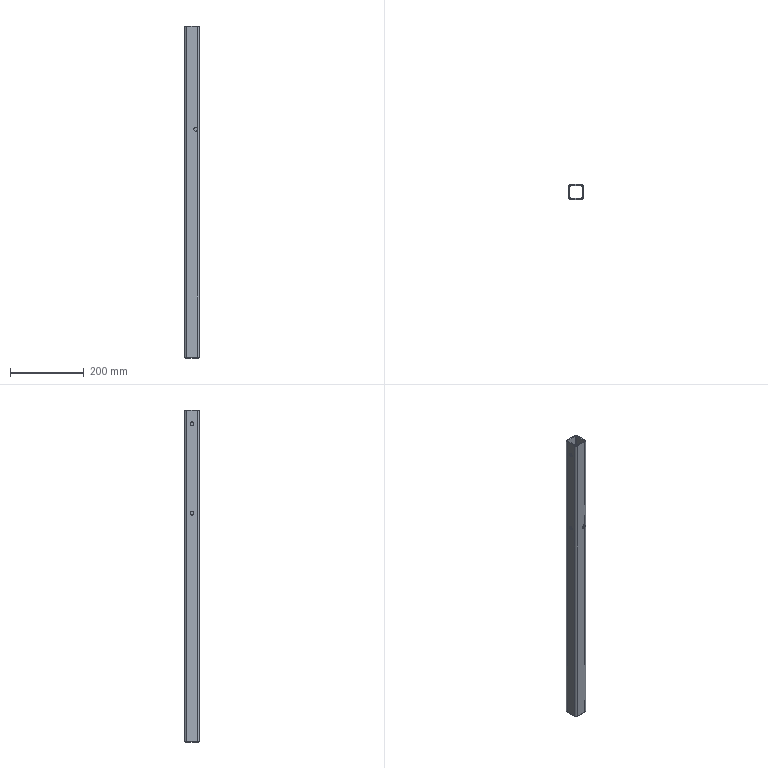Part | STEP file | DIN 59 410 - 40x40x2.9-1000_1 | 1 solid | 29 faces | box 40 x 40 x 900 mm | volume 366857 mm3 | plane 14 | cylinder 11 | cone 4 | commonest cylinder face diameters 5.8 x4 11.6 x4 10 x3